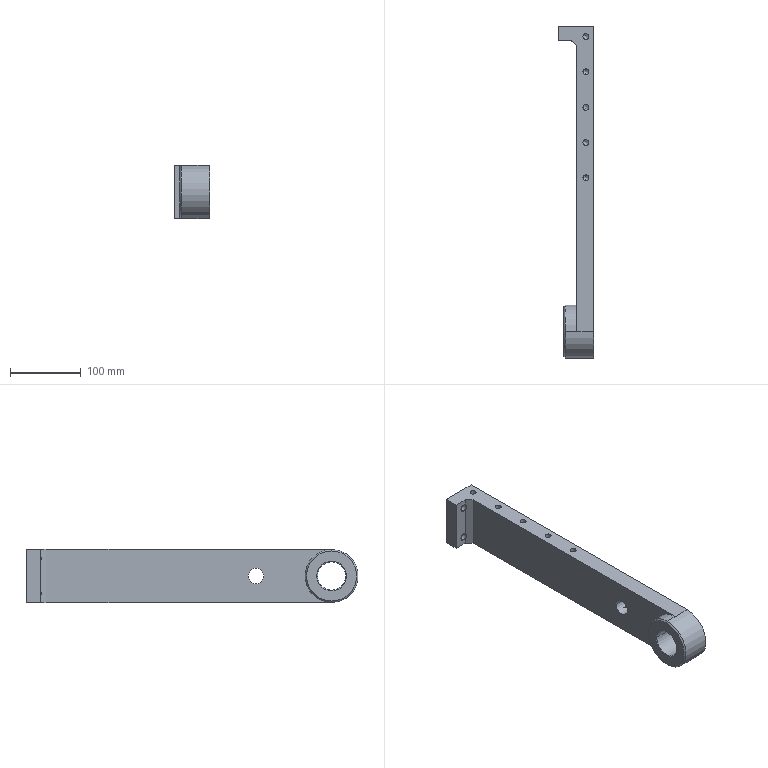Part | SolidWorks | features BaseBody 1 | 1 solid | 77 faces | box 50 x 470 x 75 mm | volume 866067 mm3 | cylinder 36 | cone 32 | plane 9 | commonest cylinder face diameters 8.376 x26 10.106 x4 22 x2 40 x2 75 x2